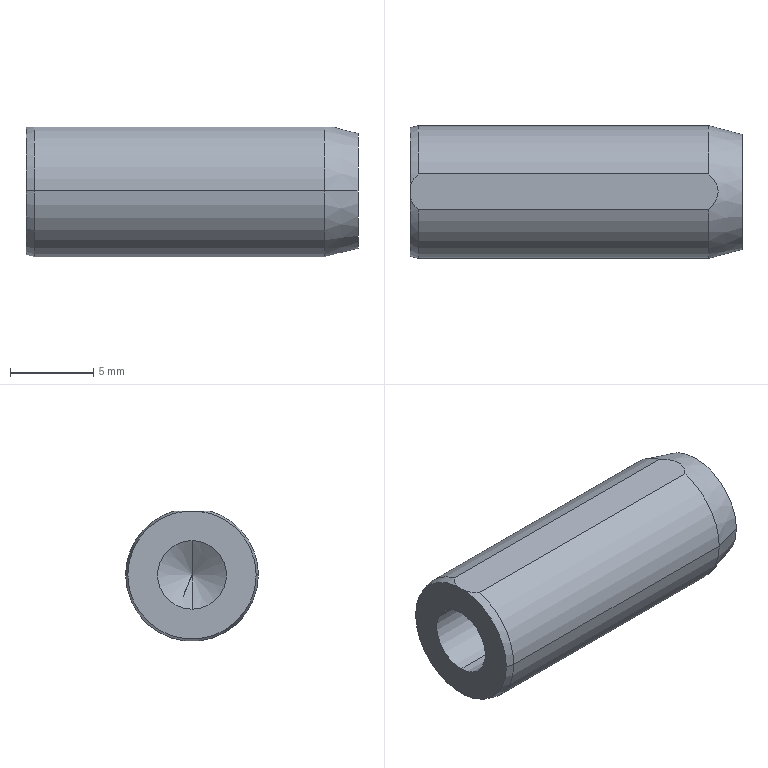Part | STEP file | MSTMS8-20-Part-1 | 1 solid | 15 faces | box 20 x 8 x 7.85 mm | volume 874.766 mm3 | cone 7 | cylinder 5 | plane 3 | commonest cylinder face diameters 8 x3 4.134 x2
STEP:
#1=CARTESIAN_POINT('',(0.,0.,0.));
#2=DIRECTION('',(0.,0.,1.));
#3=DIRECTION('',(1.,0.,0.));
#4=AXIS2_PLACEMENT_3D('',#1,#2,#3);
#5=CARTESIAN_POINT('',(-26.,-265.,-87.933));
#6=VERTEX_POINT('',#5);
#7=CARTESIAN_POINT('',(-34.,-265.,-87.933));
#8=VERTEX_POINT('',#7);
#9=CARTESIAN_POINT('',(-34.,-265.,-87.933));
#10=DIRECTION('',(-1.,0.,0.));
#11=VECTOR('',#10,1.);
#12=LINE('',#9,#11);
#13=CARTESIAN_POINT('',(-34.,-265.,-90.));
#14=DIRECTION('',(-1.,0.,0.));
#15=DIRECTION('',(0.,0.,1.));
#16=AXIS2_PLACEMENT_3D('',#13,#14,#15);
#17=CYLINDRICAL_SURFACE('',#16,2.067);
#18=CARTESIAN_POINT('',(6.283,0.));
#19=DIRECTION('',(0.,1.));
#20=VECTOR('',#19,1.);
#21=LINE('',#18,#20);
#22=(GEOMETRIC_REPRESENTATION_CONTEXT(2)PARAMETRIC_REPRESENTATION_CONTEXT()REPRESENTATION_CONTEXT('',''));
#23=DEFINITIONAL_REPRESENTATION('',(#21),#22);
#24=PCURVE('',#17,#23);
#25=CARTESIAN_POINT('',(-34.,-265.,-90.));
#26=DIRECTION('',(-1.,0.,0.));
#27=DIRECTION('',(0.,0.,1.));
#28=AXIS2_PLACEMENT_3D('',#25,#26,#27);
#29=CYLINDRICAL_SURFACE('',#28,2.067);
#30=CARTESIAN_POINT('',(0.,0.));
#31=DIRECTION('',(0.,1.));
#32=VECTOR('',#31,1.);
#33=LINE('',#30,#32);
#34=(GEOMETRIC_REPRESENTATION_CONTEXT(2)PARAMETRIC_REPRESENTATION_CONTEXT()REPRESENTATION_CONTEXT('',''));
#35=DEFINITIONAL_REPRESENTATION('',(#33),#34);
#36=PCURVE('',#29,#35);
#37=SURFACE_CURVE('',#12,(#24,#36),.PCURVE_S1.);
#38=EDGE_CURVE('',#6,#8,#37,.T.);
#39=ORIENTED_EDGE('',*,*,#38,.T.);
#40=CARTESIAN_POINT('',(-34.,-265.,-92.067));
#41=VERTEX_POINT('',#40);
#42=CARTESIAN_POINT('',(-34.,-265.,-90.));
#43=DIRECTION('',(-1.,0.,0.));
#44=DIRECTION('',(0.,0.,1.));
#45=AXIS2_PLACEMENT_3D('',#42,#43,#44);
#46=CIRCLE('',#45,2.067);
#47=CARTESIAN_POINT('',(0.,0.));
#48=DIRECTION('',(1.,0.));
#49=VECTOR('',#48,1.);
#50=LINE('',#47,#49);
#51=(GEOMETRIC_REPRESENTATION_CONTEXT(2)PARAMETRIC_REPRESENTATION_CONTEXT()REPRESENTATION_CONTEXT('',''));
#52=DEFINITIONAL_REPRESENTATION('',(#50),#51);
#53=PCURVE('',#17,#52);
#54=CARTESIAN_POINT('',(-34.,-265.,-90.));
#55=DIRECTION('',(-1.,0.,0.));
#56=DIRECTION('',(0.,-1.,0.));
#57=AXIS2_PLACEMENT_3D('',#54,#55,#56);
#58=PLANE('',#57);
#59=CARTESIAN_POINT('',(0.,0.));
#60=DIRECTION('',(0.,1.));
#61=AXIS2_PLACEMENT_2D('',#59,#60);
#62=CIRCLE('',#61,2.067);
#63=(GEOMETRIC_REPRESENTATION_CONTEXT(2)PARAMETRIC_REPRESENTATION_CONTEXT()REPRESENTATION_CONTEXT('',''));
#64=DEFINITIONAL_REPRESENTATION('',(#62),#63);
#65=PCURVE('',#58,#64);
#66=SURFACE_CURVE('',#46,(#53,#65),.PCURVE_S1.);
#67=EDGE_CURVE('',#41,#8,#66,.T.);
#68=ORIENTED_EDGE('',*,*,#67,.F.);
#69=CARTESIAN_POINT('',(-26.,-265.,-92.067));
#70=VERTEX_POINT('',#69);
#71=CARTESIAN_POINT('',(-34.,-265.,-92.067));
#72=DIRECTION('',(-1.,0.,0.));
#73=VECTOR('',#72,1.);
#74=LINE('',#71,#73);
#75=CARTESIAN_POINT('',(3.142,0.));
#76=DIRECTION('',(0.,1.));
#77=VECTOR('',#76,1.);
#78=LINE('',#75,#77);
#79=(GEOMETRIC_REPRESENTATION_CONTEXT(2)PARAMETRIC_REPRESENTATION_CONTEXT()REPRESENTATION_CONTEXT('',''));
#80=DEFINITIONAL_REPRESENTATION('',(#78),#79);
#81=PCURVE('',#17,#80);
#82=CARTESIAN_POINT('',(3.142,0.));
#83=DIRECTION('',(0.,1.));
#84=VECTOR('',#83,1.);
#85=LINE('',#82,#84);
#86=(GEOMETRIC_REPRESENTATION_CONTEXT(2)PARAMETRIC_REPRESENTATION_CONTEXT()REPRESENTATION_CONTEXT('',''));
#87=DEFINITIONAL_REPRESENTATION('',(#85),#86);
#88=PCURVE('',#29,#87);
#89=SURFACE_CURVE('',#74,(#81,#88),.PCURVE_S1.);
#90=EDGE_CURVE('',#70,#41,#89,.T.);
#91=ORIENTED_EDGE('',*,*,#90,.F.);
#92=CARTESIAN_POINT('',(-26.,-265.,-90.));
#93=DIRECTION('',(-1.,0.,0.));
#94=DIRECTION('',(0.,0.,1.));
#95=AXIS2_PLACEMENT_3D('',#92,#93,#94);
#96=CIRCLE('',#95,2.067);
#97=CARTESIAN_POINT('',(0.,-8.));
#98=DIRECTION('',(1.,0.));
#99=VECTOR('',#98,1.);
#100=LINE('',#97,#99);
#101=(GEOMETRIC_REPRESENTATION_CONTEXT(2)PARAMETRIC_REPRESENTATION_CONTEXT()REPRESENTATION_CONTEXT('',''));
#102=DEFINITIONAL_REPRESENTATION('',(#100),#101);
#103=PCURVE('',#17,#102);
#104=CARTESIAN_POINT('',(-26.,-265.,-90.));
#105=DIRECTION('',(-1.,0.,0.));
#106=DIRECTION('',(0.,0.,1.));
#107=AXIS2_PLACEMENT_3D('',#104,#105,#106);
#108=CONICAL_SURFACE('',#107,2.067,1.03);
#109=CARTESIAN_POINT('',(0.,0.));
#110=DIRECTION('',(1.,0.));
#111=VECTOR('',#110,1.);
#112=LINE('',#109,#111);
#113=(GEOMETRIC_REPRESENTATION_CONTEXT(2)PARAMETRIC_REPRESENTATION_CONTEXT()REPRESENTATION_CONTEXT('',''));
#114=DEFINITIONAL_REPRESENTATION('',(#112),#113);
#115=PCURVE('',#108,#114);
#116=SURFACE_CURVE('',#96,(#103,#115),.PCURVE_S1.);
#117=EDGE_CURVE('',#70,#6,#116,.T.);
#118=ORIENTED_EDGE('',*,*,#117,.T.);
#119=EDGE_LOOP('',(#39,#68,#91,#118));
#120=FACE_BOUND('',#119,.F.);
#121=ADVANCED_FACE('',(#120),#17,.F.);
#122=ORIENTED_EDGE('',*,*,#117,.F.);
#123=CARTESIAN_POINT('',(-24.758,-265.,-90.));
#124=VERTEX_POINT('',#123);
#125=CARTESIAN_POINT('',(-26.,-265.,-92.067));
#126=DIRECTION('',(-0.515,0.,-0.8572));
#127=VECTOR('',#126,1.);
#128=LINE('',#125,#127);
#129=CARTESIAN_POINT('',(3.142,0.));
#130=DIRECTION('',(0.,1.));
#131=VECTOR('',#130,1.);
#132=LINE('',#129,#131);
#133=(GEOMETRIC_REPRESENTATION_CONTEXT(2)PARAMETRIC_REPRESENTATION_CONTEXT()REPRESENTATION_CONTEXT('',''));
#134=DEFINITIONAL_REPRESENTATION('',(#132),#133);
#135=PCURVE('',#108,#134);
#136=CARTESIAN_POINT('',(-26.,-265.,-90.));
#137=DIRECTION('',(-1.,0.,0.));
#138=DIRECTION('',(0.,0.,1.));
#139=AXIS2_PLACEMENT_3D('',#136,#137,#138);
#140=CONICAL_SURFACE('',#139,2.067,1.03);
#141=CARTESIAN_POINT('',(3.142,0.));
#142=DIRECTION('',(0.,1.));
#143=VECTOR('',#142,1.);
#144=LINE('',#141,#143);
#145=(GEOMETRIC_REPRESENTATION_CONTEXT(2)PARAMETRIC_REPRESENTATION_CONTEXT()REPRESENTATION_CONTEXT('',''));
#146=DEFINITIONAL_REPRESENTATION('',(#144),#145);
#147=PCURVE('',#140,#146);
#148=SURFACE_CURVE('',#128,(#135,#147),.PCURVE_S1.);
#149=EDGE_CURVE('',#124,#70,#148,.T.);
#150=ORIENTED_EDGE('',*,*,#149,.F.);
#151=CARTESIAN_POINT('',(-26.,-265.,-87.933));
#152=DIRECTION('',(-0.515,0.,0.8572));
#153=VECTOR('',#152,1.);
#154=LINE('',#151,#153);
#155=CARTESIAN_POINT('',(6.283,0.));
#156=DIRECTION('',(0.,1.));
#157=VECTOR('',#156,1.);
#158=LINE('',#155,#157);
#159=(GEOMETRIC_REPRESENTATION_CONTEXT(2)PARAMETRIC_REPRESENTATION_CONTEXT()REPRESENTATION_CONTEXT('',''));
#160=DEFINITIONAL_REPRESENTATION('',(#158),#159);
#161=PCURVE('',#108,#160);
#162=CARTESIAN_POINT('',(0.,0.));
#163=DIRECTION('',(0.,1.));
#164=VECTOR('',#163,1.);
#165=LINE('',#162,#164);
#166=(GEOMETRIC_REPRESENTATION_CONTEXT(2)PARAMETRIC_REPRESENTATION_CONTEXT()REPRESENTATION_CONTEXT('',''));
#167=DEFINITIONAL_REPRESENTATION('',(#165),#166);
#168=PCURVE('',#140,#167);
#169=SURFACE_CURVE('',#154,(#161,#168),.PCURVE_S1.);
#170=EDGE_CURVE('',#124,#6,#169,.T.);
#171=ORIENTED_EDGE('',*,*,#170,.T.);
#172=EDGE_LOOP('',(#122,#150,#171));
#173=FACE_BOUND('',#172,.F.);
#174=ADVANCED_FACE('',(#173),#108,.F.);
#175=CARTESIAN_POINT('',(-14.,-261.536,-90.));
#176=VERTEX_POINT('',#175);
#177=CARTESIAN_POINT('',(-14.,-268.464,-90.));
#178=VERTEX_POINT('',#177);
#179=CARTESIAN_POINT('',(-14.,-265.,-90.));
#180=DIRECTION('',(1.,0.,0.));
#181=DIRECTION('',(0.,1.,0.));
#182=AXIS2_PLACEMENT_3D('',#179,#180,#181);
#183=CIRCLE('',#182,3.464);
#184=CARTESIAN_POINT('',(-14.,-265.,-90.));
#185=DIRECTION('',(-1.,0.,0.));
#186=DIRECTION('',(0.,-1.,0.));
#187=AXIS2_PLACEMENT_3D('',#184,#185,#186);
#188=CONICAL_SURFACE('',#187,3.464,0.2618);
#189=CARTESIAN_POINT('',(3.142,0.));
#190=DIRECTION('',(-1.,0.));
#191=VECTOR('',#190,1.);
#192=LINE('',#189,#191);
#193=(GEOMETRIC_REPRESENTATION_CONTEXT(2)PARAMETRIC_REPRESENTATION_CONTEXT()REPRESENTATION_CONTEXT('',''));
#194=DEFINITIONAL_REPRESENTATION('',(#192),#193);
#195=PCURVE('',#188,#194);
#196=CARTESIAN_POINT('',(-14.,-265.,-90.));
#197=DIRECTION('',(1.,0.,0.));
#198=DIRECTION('',(0.,1.,0.));
#199=AXIS2_PLACEMENT_3D('',#196,#197,#198);
#200=PLANE('',#199);
#201=CARTESIAN_POINT('',(0.,0.));
#202=DIRECTION('',(1.,0.));
#203=AXIS2_PLACEMENT_2D('',#201,#202);
#204=CIRCLE('',#203,3.464);
#205=(GEOMETRIC_REPRESENTATION_CONTEXT(2)PARAMETRIC_REPRESENTATION_CONTEXT()REPRESENTATION_CONTEXT('',''));
#206=DEFINITIONAL_REPRESENTATION('',(#204),#205);
#207=PCURVE('',#200,#206);
#208=SURFACE_CURVE('',#183,(#195,#207),.PCURVE_S1.);
#209=EDGE_CURVE('',#176,#178,#208,.T.);
#210=ORIENTED_EDGE('',*,*,#209,.F.);
#211=CARTESIAN_POINT('',(-16.,-261.,-90.));
#212=VERTEX_POINT('',#211);
#213=CARTESIAN_POINT('',(-14.,-261.536,-90.));
#214=DIRECTION('',(-0.9659,0.2588,0.));
#215=VECTOR('',#214,1.);
#216=LINE('',#213,#215);
#217=CARTESIAN_POINT('',(3.142,0.));
#218=DIRECTION('',(0.,1.));
#219=VECTOR('',#218,1.);
#220=LINE('',#217,#219);
#221=(GEOMETRIC_REPRESENTATION_CONTEXT(2)PARAMETRIC_REPRESENTATION_CONTEXT()REPRESENTATION_CONTEXT('',''));
#222=DEFINITIONAL_REPRESENTATION('',(#220),#221);
#223=PCURVE('',#188,#222);
#224=CARTESIAN_POINT('',(-14.,-265.,-90.));
#225=DIRECTION('',(-1.,0.,0.));
#226=DIRECTION('',(0.,-1.,0.));
#227=AXIS2_PLACEMENT_3D('',#224,#225,#226);
#228=CONICAL_SURFACE('',#227,3.464,0.2618);
#229=CARTESIAN_POINT('',(3.142,0.));
#230=DIRECTION('',(0.,1.));
#231=VECTOR('',#230,1.);
#232=LINE('',#229,#231);
#233=(GEOMETRIC_REPRESENTATION_CONTEXT(2)PARAMETRIC_REPRESENTATION_CONTEXT()REPRESENTATION_CONTEXT('',''));
#234=DEFINITIONAL_REPRESENTATION('',(#232),#233);
#235=PCURVE('',#228,#234);
#236=SURFACE_CURVE('',#216,(#223,#235),.PCURVE_S1.);
#237=EDGE_CURVE('',#176,#212,#236,.T.);
#238=ORIENTED_EDGE('',*,*,#237,.T.);
#239=CARTESIAN_POINT('',(-16.,-263.915,-86.15));
#240=VERTEX_POINT('',#239);
#241=CARTESIAN_POINT('',(-16.,-265.,-90.));
#242=DIRECTION('',(1.,0.,0.));
#243=DIRECTION('',(0.,1.,0.));
#244=AXIS2_PLACEMENT_3D('',#241,#242,#243);
#245=CIRCLE('',#244,4.);
#246=CARTESIAN_POINT('',(3.142,2.));
#247=DIRECTION('',(-1.,0.));
#248=VECTOR('',#247,1.);
#249=LINE('',#246,#248);
#250=(GEOMETRIC_REPRESENTATION_CONTEXT(2)PARAMETRIC_REPRESENTATION_CONTEXT()REPRESENTATION_CONTEXT('',''));
#251=DEFINITIONAL_REPRESENTATION('',(#249),#250);
#252=PCURVE('',#188,#251);
#253=CARTESIAN_POINT('',(-14.,-265.,-90.));
#254=DIRECTION('',(1.,0.,0.));
#255=DIRECTION('',(0.,1.,0.));
#256=AXIS2_PLACEMENT_3D('',#253,#254,#255);
#257=CYLINDRICAL_SURFACE('',#256,4.);
#258=CARTESIAN_POINT('',(0.,-2.));
#259=DIRECTION('',(1.,0.));
#260=VECTOR('',#259,1.);
#261=LINE('',#258,#260);
#262=(GEOMETRIC_REPRESENTATION_CONTEXT(2)PARAMETRIC_REPRESENTATION_CONTEXT()REPRESENTATION_CONTEXT('',''));
#263=DEFINITIONAL_REPRESENTATION('',(#261),#262);
#264=PCURVE('',#257,#263);
#265=SURFACE_CURVE('',#245,(#252,#264),.PCURVE_S1.);
#266=EDGE_CURVE('',#212,#240,#265,.T.);
#267=ORIENTED_EDGE('',*,*,#266,.T.);
#268=CARTESIAN_POINT('',(-16.,-266.085,-86.15));
#269=VERTEX_POINT('',#268);
#270=CARTESIAN_POINT('',(-16.,-266.085,-86.15));
#271=CARTESIAN_POINT('',(-15.853,-265.94,-86.15));
#272=CARTESIAN_POINT('',(-15.716,-265.778,-86.15));
#273=CARTESIAN_POINT('',(-15.508,-265.416,-86.15));
#274=CARTESIAN_POINT('',(-15.44,-265.21,-86.15));
#275=CARTESIAN_POINT('',(-15.44,-264.789,-86.15));
#276=CARTESIAN_POINT('',(-15.508,-264.584,-86.15));
#277=CARTESIAN_POINT('',(-15.663,-264.313,-86.15));
#278=CARTESIAN_POINT('',(-15.724,-264.227,-86.15));
#279=CARTESIAN_POINT('',(-15.856,-264.064,-86.15));
#280=CARTESIAN_POINT('',(-15.926,-263.988,-86.15));
#281=CARTESIAN_POINT('',(-16.,-263.915,-86.15));
#282=B_SPLINE_CURVE_WITH_KNOTS('',3,(#270,#271,#272,#273,#274,#275,#276,#277,#278,#279,#280,#281),.UNSPECIFIED.,.F.,.F.,(4,2,2,2,2,4),(0.001238,0.001854,0.00247,0.003086,0.003394,0.003702),.UNSPECIFIED.);
#283=CARTESIAN_POINT('',(1.296,2.));
#284=CARTESIAN_POINT('',(1.302,1.973));
#285=CARTESIAN_POINT('',(1.315,1.921));
#286=CARTESIAN_POINT('',(1.336,1.844));
#287=CARTESIAN_POINT('',(1.358,1.771));
#288=CARTESIAN_POINT('',(1.38,1.703));
#289=CARTESIAN_POINT('',(1.404,1.64));
#290=CARTESIAN_POINT('',(1.429,1.583));
#291=CARTESIAN_POINT('',(1.456,1.534));
#292=CARTESIAN_POINT('',(1.483,1.494));
#293=CARTESIAN_POINT('',(1.512,1.464));
#294=CARTESIAN_POINT('',(1.541,1.445));
#295=CARTESIAN_POINT('',(1.571,1.438));
#296=CARTESIAN_POINT('',(1.601,1.445));
#297=CARTESIAN_POINT('',(1.63,1.464));
#298=CARTESIAN_POINT('',(1.658,1.494));
#299=CARTESIAN_POINT('',(1.686,1.534));
#300=CARTESIAN_POINT('',(1.712,1.583));
#301=CARTESIAN_POINT('',(1.737,1.64));
#302=CARTESIAN_POINT('',(1.761,1.703));
#303=CARTESIAN_POINT('',(1.784,1.772));
#304=CARTESIAN_POINT('',(1.806,1.844));
#305=CARTESIAN_POINT('',(1.826,1.92));
#306=CARTESIAN_POINT('',(1.839,1.973));
#307=CARTESIAN_POINT('',(1.846,2.));
#308=B_SPLINE_CURVE_WITH_KNOTS('',3,(#283,#284,#285,#286,#287,#288,#289,#290,#291,#292,#293,#294,#295,#296,#297,#298,#299,#300,#301,#302,#303,#304,#305,#306,#307),.UNSPECIFIED.,.F.,.F.,(4,1,1,1,1,1,1,1,1,1,1,1,1,1,1,1,1,1,1,1,1,1,4),(0.001238,0.00135,0.001462,0.001574,0.001686,0.001798,0.00191,0.002022,0.002134,0.002246,0.002358,0.00247,0.002582,0.002694,0.002806,0.002918,0.00303,0.003142,0.003254,0.003366,0.003478,0.00359,0.003702),.QUASI_UNIFORM_KNOTS.);
#309=(GEOMETRIC_REPRESENTATION_CONTEXT(2)PARAMETRIC_REPRESENTATION_CONTEXT()REPRESENTATION_CONTEXT('',''));
#310=DEFINITIONAL_REPRESENTATION('',(#308),#309);
#311=PCURVE('',#188,#310);
#312=CARTESIAN_POINT('',(-34.,-263.915,-86.15));
#313=DIRECTION('',(0.,0.,-1.));
#314=DIRECTION('',(-1.,0.,0.));
#315=AXIS2_PLACEMENT_3D('',#312,#313,#314);
#316=PLANE('',#315);
#317=CARTESIAN_POINT('',(-18.,-2.17));
#318=CARTESIAN_POINT('',(-18.147,-2.025));
#319=CARTESIAN_POINT('',(-18.284,-1.864));
#320=CARTESIAN_POINT('',(-18.492,-1.501));
#321=CARTESIAN_POINT('',(-18.56,-1.295));
#322=CARTESIAN_POINT('',(-18.56,-0.8744));
#323=CARTESIAN_POINT('',(-18.492,-0.6696));
#324=CARTESIAN_POINT('',(-18.337,-0.3981));
#325=CARTESIAN_POINT('',(-18.276,-0.3116));
#326=CARTESIAN_POINT('',(-18.144,-0.1493));
#327=CARTESIAN_POINT('',(-18.074,-0.07297));
#328=CARTESIAN_POINT('',(-18.,0.));
#329=B_SPLINE_CURVE_WITH_KNOTS('',3,(#317,#318,#319,#320,#321,#322,#323,#324,#325,#326,#327,#328),.UNSPECIFIED.,.F.,.F.,(4,2,2,2,2,4),(0.001238,0.001854,0.00247,0.003086,0.003394,0.003702),.UNSPECIFIED.);
#330=(GEOMETRIC_REPRESENTATION_CONTEXT(2)PARAMETRIC_REPRESENTATION_CONTEXT()REPRESENTATION_CONTEXT('',''));
#331=DEFINITIONAL_REPRESENTATION('',(#329),#330);
#332=PCURVE('',#316,#331);
#333=SURFACE_CURVE('',#282,(#311,#332),.PCURVE_S1.);
#334=EDGE_CURVE('',#269,#240,#333,.T.);
#335=ORIENTED_EDGE('',*,*,#334,.F.);
#336=CARTESIAN_POINT('',(-16.,-269.,-90.));
#337=VERTEX_POINT('',#336);
#338=CARTESIAN_POINT('',(-16.,-265.,-90.));
#339=DIRECTION('',(1.,0.,0.));
#340=DIRECTION('',(0.,1.,0.));
#341=AXIS2_PLACEMENT_3D('',#338,#339,#340);
#342=CIRCLE('',#341,4.);
#343=CARTESIAN_POINT('',(3.142,2.));
#344=DIRECTION('',(-1.,0.));
#345=VECTOR('',#344,1.);
#346=LINE('',#343,#345);
#347=(GEOMETRIC_REPRESENTATION_CONTEXT(2)PARAMETRIC_REPRESENTATION_CONTEXT()REPRESENTATION_CONTEXT('',''));
#348=DEFINITIONAL_REPRESENTATION('',(#346),#347);
#349=PCURVE('',#188,#348);
#350=CARTESIAN_POINT('',(-14.,-265.,-90.));
#351=DIRECTION('',(1.,0.,0.));
#352=DIRECTION('',(0.,1.,0.));
#353=AXIS2_PLACEMENT_3D('',#350,#351,#352);
#354=CYLINDRICAL_SURFACE('',#353,4.);
#355=CARTESIAN_POINT('',(0.,-2.));
#356=DIRECTION('',(1.,0.));
#357=VECTOR('',#356,1.);
#358=LINE('',#355,#357);
#359=(GEOMETRIC_REPRESENTATION_CONTEXT(2)PARAMETRIC_REPRESENTATION_CONTEXT()REPRESENTATION_CONTEXT('',''));
#360=DEFINITIONAL_REPRESENTATION('',(#358),#359);
#361=PCURVE('',#354,#360);
#362=SURFACE_CURVE('',#342,(#349,#361),.PCURVE_S1.);
#363=EDGE_CURVE('',#269,#337,#362,.T.);
#364=ORIENTED_EDGE('',*,*,#363,.T.);
#365=CARTESIAN_POINT('',(-14.,-268.464,-90.));
#366=DIRECTION('',(-0.9659,-0.2588,0.));
#367=VECTOR('',#366,1.);
#368=LINE('',#365,#367);
#369=CARTESIAN_POINT('',(0.,0.));
#370=DIRECTION('',(0.,1.));
#371=VECTOR('',#370,1.);
#372=LINE('',#369,#371);
#373=(GEOMETRIC_REPRESENTATION_CONTEXT(2)PARAMETRIC_REPRESENTATION_CONTEXT()REPRESENTATION_CONTEXT('',''));
#374=DEFINITIONAL_REPRESENTATION('',(#372),#373);
#375=PCURVE('',#188,#374);
#376=CARTESIAN_POINT('',(6.283,0.));
#377=DIRECTION('',(0.,1.));
#378=VECTOR('',#377,1.);
#379=LINE('',#376,#378);
#380=(GEOMETRIC_REPRESENTATION_CONTEXT(2)PARAMETRIC_REPRESENTATION_CONTEXT()REPRESENTATION_CONTEXT('',''));
#381=DEFINITIONAL_REPRESENTATION('',(#379),#380);
#382=PCURVE('',#228,#381);
#383=SURFACE_CURVE('',#368,(#375,#382),.PCURVE_S1.);
#384=EDGE_CURVE('',#178,#337,#383,.T.);
#385=ORIENTED_EDGE('',*,*,#384,.F.);
#386=EDGE_LOOP('',(#210,#238,#267,#335,#364,#385));
#387=FACE_BOUND('',#386,.T.);
#388=ADVANCED_FACE('',(#387),#188,.T.);
#389=CARTESIAN_POINT('',(-33.5,-266.085,-86.15));
#390=VERTEX_POINT('',#389);
#391=CARTESIAN_POINT('',(-33.5,-269.,-90.));
#392=VERTEX_POINT('',#391);
#393=CARTESIAN_POINT('',(-33.5,-265.,-90.));
#394=DIRECTION('',(1.,0.,0.));
#395=DIRECTION('',(0.,1.,0.));
#396=AXIS2_PLACEMENT_3D('',#393,#394,#395);
#397=CIRCLE('',#396,4.);
#398=CARTESIAN_POINT('',(0.,-19.5));
#399=DIRECTION('',(1.,0.));
#400=VECTOR('',#399,1.);
#401=LINE('',#398,#400);
#402=(GEOMETRIC_REPRESENTATION_CONTEXT(2)PARAMETRIC_REPRESENTATION_CONTEXT()REPRESENTATION_CONTEXT('',''));
#403=DEFINITIONAL_REPRESENTATION('',(#401),#402);
#404=PCURVE('',#354,#403);
#405=CARTESIAN_POINT('',(-33.5,-265.,-90.));
#406=DIRECTION('',(1.,0.,0.));
#407=DIRECTION('',(0.,1.,0.));
#408=AXIS2_PLACEMENT_3D('',#405,#406,#407);
#409=CONICAL_SURFACE('',#408,4.,0.2618);
#410=CARTESIAN_POINT('',(0.,0.));
#411=DIRECTION('',(1.,0.));
#412=VECTOR('',#411,1.);
#413=LINE('',#410,#412);
#414=(GEOMETRIC_REPRESENTATION_CONTEXT(2)PARAMETRIC_REPRESENTATION_CONTEXT()REPRESENTATION_CONTEXT('',''));
#415=DEFINITIONAL_REPRESENTATION('',(#413),#414);
#416=PCURVE('',#409,#415);
#417=SURFACE_CURVE('',#397,(#404,#416),.PCURVE_S1.);
#418=EDGE_CURVE('',#390,#392,#417,.T.);
#419=ORIENTED_EDGE('',*,*,#418,.T.);
#420=CARTESIAN_POINT('',(-14.,-269.,-90.));
#421=DIRECTION('',(1.,0.,0.));
#422=VECTOR('',#421,1.);
#423=LINE('',#420,#422);
#424=CARTESIAN_POINT('',(3.142,0.));
#425=DIRECTION('',(0.,1.));
#426=VECTOR('',#425,1.);
#427=LINE('',#424,#426);
#428=(GEOMETRIC_REPRESENTATION_CONTEXT(2)PARAMETRIC_REPRESENTATION_CONTEXT()REPRESENTATION_CONTEXT('',''));
#429=DEFINITIONAL_REPRESENTATION('',(#427),#428);
#430=PCURVE('',#354,#429);
#431=CARTESIAN_POINT('',(-14.,-265.,-90.));
#432=DIRECTION('',(1.,0.,0.));
#433=DIRECTION('',(0.,1.,0.));
#434=AXIS2_PLACEMENT_3D('',#431,#432,#433);
#435=CYLINDRICAL_SURFACE('',#434,4.);
#436=CARTESIAN_POINT('',(3.142,0.));
#437=DIRECTION('',(0.,1.));
#438=VECTOR('',#437,1.);
#439=LINE('',#436,#438);
#440=(GEOMETRIC_REPRESENTATION_CONTEXT(2)PARAMETRIC_REPRESENTATION_CONTEXT()REPRESENTATION_CONTEXT('',''));
#441=DEFINITIONAL_REPRESENTATION('',(#439),#440);
#442=PCURVE('',#435,#441);
#443=SURFACE_CURVE('',#423,(#430,#442),.PCURVE_S1.);
#444=EDGE_CURVE('',#392,#337,#443,.T.);
#445=ORIENTED_EDGE('',*,*,#444,.T.);
#446=ORIENTED_EDGE('',*,*,#363,.F.);
#447=CARTESIAN_POINT('',(-34.,-266.085,-86.15));
#448=DIRECTION('',(1.,0.,0.));
#449=VECTOR('',#448,1.);
#450=LINE('',#447,#449);
#451=CARTESIAN_POINT('',(1.846,-20.));
#452=DIRECTION('',(0.,1.));
#453=VECTOR('',#452,1.);
#454=LINE('',#451,#453);
#455=(GEOMETRIC_REPRESENTATION_CONTEXT(2)PARAMETRIC_REPRESENTATION_CONTEXT()REPRESENTATION_CONTEXT('',''));
#456=DEFINITIONAL_REPRESENTATION('',(#454),#455);
#457=PCURVE('',#354,#456);
#458=CARTESIAN_POINT('',(0.,-2.17));
#459=DIRECTION('',(-1.,0.));
#460=VECTOR('',#459,1.);
#461=LINE('',#458,#460);
#462=(GEOMETRIC_REPRESENTATION_CONTEXT(2)PARAMETRIC_REPRESENTATION_CONTEXT()REPRESENTATION_CONTEXT('',''));
#463=DEFINITIONAL_REPRESENTATION('',(#461),#462);
#464=PCURVE('',#316,#463);
#465=SURFACE_CURVE('',#450,(#457,#464),.PCURVE_S1.);
#466=EDGE_CURVE('',#390,#269,#465,.T.);
#467=ORIENTED_EDGE('',*,*,#466,.F.);
#468=EDGE_LOOP('',(#419,#445,#446,#467));
#469=FACE_BOUND('',#468,.T.);
#470=ADVANCED_FACE('',(#469),#354,.T.);
#471=ORIENTED_EDGE('',*,*,#444,.F.);
#472=CARTESIAN_POINT('',(-33.5,-261.,-90.));
#473=VERTEX_POINT('',#472);
#474=CARTESIAN_POINT('',(-33.5,-265.,-90.));
#475=DIRECTION('',(1.,0.,0.));
#476=DIRECTION('',(0.,1.,0.));
#477=AXIS2_PLACEMENT_3D('',#474,#475,#476);
#478=CIRCLE('',#477,4.);
#479=CARTESIAN_POINT('',(0.,-19.5));
#480=DIRECTION('',(1.,0.));
#481=VECTOR('',#480,1.);
#482=LINE('',#479,#481);
#483=(GEOMETRIC_REPRESENTATION_CONTEXT(2)PARAMETRIC_REPRESENTATION_CONTEXT()REPRESENTATION_CONTEXT('',''));
#484=DEFINITIONAL_REPRESENTATION('',(#482),#483);
#485=PCURVE('',#435,#484);
#486=CARTESIAN_POINT('',(-33.5,-265.,-90.));
#487=DIRECTION('',(1.,0.,0.));
#488=DIRECTION('',(0.,1.,0.));
#489=AXIS2_PLACEMENT_3D('',#486,#487,#488);
#490=CONICAL_SURFACE('',#489,4.,0.2618);
#491=CARTESIAN_POINT('',(0.,0.));
#492=DIRECTION('',(1.,0.));
#493=VECTOR('',#492,1.);
#494=LINE('',#491,#493);
#495=(GEOMETRIC_REPRESENTATION_CONTEXT(2)PARAMETRIC_REPRESENTATION_CONTEXT()REPRESENTATION_CONTEXT('',''));
#496=DEFINITIONAL_REPRESENTATION('',(#494),#495);
#497=PCURVE('',#490,#496);
#498=SURFACE_CURVE('',#478,(#485,#497),.PCURVE_S1.);
#499=EDGE_CURVE('',#392,#473,#498,.T.);
#500=ORIENTED_EDGE('',*,*,#499,.T.);
#501=CARTESIAN_POINT('',(-14.,-261.,-90.));
#502=DIRECTION('',(1.,0.,0.));
#503=VECTOR('',#502,1.);
#504=LINE('',#501,#503);
#505=CARTESIAN_POINT('',(6.283,0.));
#506=DIRECTION('',(0.,1.));
#507=VECTOR('',#506,1.);
#508=LINE('',#505,#507);
#509=(GEOMETRIC_REPRESENTATION_CONTEXT(2)PARAMETRIC_REPRESENTATION_CONTEXT()REPRESENTATION_CONTEXT('',''));
#510=DEFINITIONAL_REPRESENTATION('',(#508),#509);
#511=PCURVE('',#435,#510);
#512=CARTESIAN_POINT('',(0.,0.));
#513=DIRECTION('',(0.,1.));
#514=VECTOR('',#513,1.);
#515=LINE('',#512,#514);
#516=(GEOMETRIC_REPRESENTATION_CONTEXT(2)PARAMETRIC_REPRESENTATION_CONTEXT()REPRESENTATION_CONTEXT('',''));
#517=DEFINITIONAL_REPRESENTATION('',(#515),#516);
#518=PCURVE('',#257,#517);
#519=SURFACE_CURVE('',#504,(#511,#518),.PCURVE_S1.);
#520=EDGE_CURVE('',#473,#212,#519,.T.);
#521=ORIENTED_EDGE('',*,*,#520,.T.);
#522=CARTESIAN_POINT('',(-16.,-265.,-90.));
#523=DIRECTION('',(1.,0.,0.));
#524=DIRECTION('',(0.,1.,0.));
#525=AXIS2_PLACEMENT_3D('',#522,#523,#524);
#526=CIRCLE('',#525,4.);
#527=CARTESIAN_POINT('',(0.,-2.));
#528=DIRECTION('',(1.,0.));
#529=VECTOR('',#528,1.);
#530=LINE('',#527,#529);
#531=(GEOMETRIC_REPRESENTATION_CONTEXT(2)PARAMETRIC_REPRESENTATION_CONTEXT()REPRESENTATION_CONTEXT('',''));
#532=DEFINITIONAL_REPRESENTATION('',(#530),#531);
#533=PCURVE('',#435,#532);
#534=CARTESIAN_POINT('',(9.425,2.));
#535=DIRECTION('',(-1.,0.));
#536=VECTOR('',#535,1.);
#537=LINE('',#534,#536);
#538=(GEOMETRIC_REPRESENTATION_CONTEXT(2)PARAMETRIC_REPRESENTATION_CONTEXT()REPRESENTATION_CONTEXT('',''));
#539=DEFINITIONAL_REPRESENTATION('',(#537),#538);
#540=PCURVE('',#228,#539);
#541=SURFACE_CURVE('',#526,(#533,#540),.PCURVE_S1.);
#542=EDGE_CURVE('',#337,#212,#541,.T.);
#543=ORIENTED_EDGE('',*,*,#542,.F.);
#544=EDGE_LOOP('',(#471,#500,#521,#543));
#545=FACE_BOUND('',#544,.T.);
#546=ADVANCED_FACE('',(#545),#435,.T.);
#547=CARTESIAN_POINT('',(-34.,-265.352,-86.15));
#548=VERTEX_POINT('',#547);
#549=CARTESIAN_POINT('',(-34.,-268.866,-90.));
#550=VERTEX_POINT('',#549);
#551=CARTESIAN_POINT('',(-34.,-265.,-90.));
#552=DIRECTION('',(1.,0.,0.));
#553=DIRECTION('',(0.,1.,0.));
#554=AXIS2_PLACEMENT_3D('',#551,#552,#553);
#555=CIRCLE('',#554,3.866);
#556=CARTESIAN_POINT('',(0.,-0.5));
#557=DIRECTION('',(1.,0.));
#558=VECTOR('',#557,1.);
#559=LINE('',#556,#558);
#560=(GEOMETRIC_REPRESENTATION_CONTEXT(2)PARAMETRIC_REPRESENTATION_CONTEXT()REPRESENTATION_CONTEXT('',''));
#561=DEFINITIONAL_REPRESENTATION('',(#559),#560);
#562=PCURVE('',#409,#561);
#563=CARTESIAN_POINT('',(-3.866,0.));
#564=CARTESIAN_POINT('',(-3.866,6.696));
#565=CARTESIAN_POINT('',(1.933,3.348));
#566=CARTESIAN_POINT('',(7.732,0.));
#567=CARTESIAN_POINT('',(1.933,-3.348));
#568=CARTESIAN_POINT('',(-3.866,-6.696));
#569=CARTESIAN_POINT('',(-3.866,0.));
#570=(BOUNDED_CURVE()B_SPLINE_CURVE(2,(#563,#564,#565,#566,#567,#568,#569),.UNSPECIFIED.,.T.,.F.)B_SPLINE_CURVE_WITH_KNOTS((1,2,2,2,2,1),(-2.094,0.,2.094,4.189,6.283,8.378),.UNSPECIFIED.)CURVE()GEOMETRIC_REPRESENTATION_ITEM()RATIONAL_B_SPLINE_CURVE((1.,0.5,1.,0.5,1.,0.5,1.))REPRESENTATION_ITEM(''));
#571=(GEOMETRIC_REPRESENTATION_CONTEXT(2)PARAMETRIC_REPRESENTATION_CONTEXT()REPRESENTATION_CONTEXT('',''));
#572=DEFINITIONAL_REPRESENTATION('',(#570),#571);
#573=PCURVE('',#58,#572);
#574=SURFACE_CURVE('',#555,(#562,#573),.PCURVE_S1.);
#575=EDGE_CURVE('',#548,#550,#574,.T.);
#576=ORIENTED_EDGE('',*,*,#575,.T.);
#577=CARTESIAN_POINT('',(-33.5,-269.,-90.));
#578=DIRECTION('',(0.9659,-0.2588,0.));
#579=VECTOR('',#578,1.);
#580=LINE('',#577,#579);
#581=CARTESIAN_POINT('',(3.142,0.));
#582=DIRECTION('',(0.,1.));
#583=VECTOR('',#582,1.);
#584=LINE('',#581,#583);
#585=(GEOMETRIC_REPRESENTATION_CONTEXT(2)PARAMETRIC_REPRESENTATION_CONTEXT()REPRESENTATION_CONTEXT('',''));
#586=DEFINITIONAL_REPRESENTATION('',(#584),#585);
#587=PCURVE('',#409,#586);
#588=CARTESIAN_POINT('',(3.142,0.));
#589=DIRECTION('',(0.,1.));
#590=VECTOR('',#589,1.);
#591=LINE('',#588,#590);
#592=(GEOMETRIC_REPRESENTATION_CONTEXT(2)PARAMETRIC_REPRESENTATION_CONTEXT()REPRESENTATION_CONTEXT('',''));
#593=DEFINITIONAL_REPRESENTATION('',(#591),#592);
#594=PCURVE('',#490,#593);
#595=SURFACE_CURVE('',#580,(#587,#594),.PCURVE_S1.);
#596=EDGE_CURVE('',#550,#392,#595,.T.);
#597=ORIENTED_EDGE('',*,*,#596,.T.);
#598=ORIENTED_EDGE('',*,*,#418,.F.);
#599=CARTESIAN_POINT('',(-34.,-265.352,-86.15));
#600=CARTESIAN_POINT('',(-33.952,-265.493,-86.15));
#601=CARTESIAN_POINT('',(-33.878,-265.626,-86.15));
#602=CARTESIAN_POINT('',(-33.706,-265.868,-86.15));
#603=CARTESIAN_POINT('',(-33.606,-265.98,-86.15));
#604=CARTESIAN_POINT('',(-33.5,-266.085,-86.15));
#605=B_SPLINE_CURVE_WITH_KNOTS('',3,(#599,#600,#601,#602,#603,#604),.UNSPECIFIED.,.F.,.F.,(4,2,4),(0.003237,0.003679,0.004122),.UNSPECIFIED.);
#606=CARTESIAN_POINT('',(1.662,-0.5));
#607=CARTESIAN_POINT('',(1.665,-0.4956));
#608=CARTESIAN_POINT('',(1.672,-0.4865));
#609=CARTESIAN_POINT('',(1.682,-0.4715));
#610=CARTESIAN_POINT('',(1.691,-0.4553));
#611=CARTESIAN_POINT('',(1.701,-0.4381));
#612=CARTESIAN_POINT('',(1.71,-0.4198));
#613=CARTESIAN_POINT('',(1.719,-0.4005));
#614=CARTESIAN_POINT('',(1.728,-0.3804));
#615=CARTESIAN_POINT('',(1.737,-0.3593));
#616=CARTESIAN_POINT('',(1.746,-0.3375));
#617=CARTESIAN_POINT('',(1.754,-0.315));
#618=CARTESIAN_POINT('',(1.763,-0.2918));
#619=CARTESIAN_POINT('',(1.771,-0.268));
#620=CARTESIAN_POINT('',(1.779,-0.2436));
#621=CARTESIAN_POINT('',(1.787,-0.2185));
#622=CARTESIAN_POINT('',(1.794,-0.1929));
#623=CARTESIAN_POINT('',(1.802,-0.1668));
#624=CARTESIAN_POINT('',(1.81,-0.1402));
#625=CARTESIAN_POINT('',(1.817,-0.113));
#626=CARTESIAN_POINT('',(1.824,-0.08541));
#627=CARTESIAN_POINT('',(1.832,-0.05736));
#628=CARTESIAN_POINT('',(1.839,-0.02891));
#629=CARTESIAN_POINT('',(1.843,-0.009676));
#630=CARTESIAN_POINT('',(1.846,0.));
#631=B_SPLINE_CURVE_WITH_KNOTS('',3,(#606,#607,#608,#609,#610,#611,#612,#613,#614,#615,#616,#617,#618,#619,#620,#621,#622,#623,#624,#625,#626,#627,#628,#629,#630),.UNSPECIFIED.,.F.,.F.,(4,1,1,1,1,1,1,1,1,1,1,1,1,1,1,1,1,1,1,1,1,1,4),(0.003237,0.003277,0.003317,0.003357,0.003398,0.003438,0.003478,0.003518,0.003559,0.003599,0.003639,0.003679,0.00372,0.00376,0.0038,0.00384,0.003881,0.003921,0.003961,0.004001,0.004042,0.004082,0.004122),.QUASI_UNIFORM_KNOTS.);
#632=(GEOMETRIC_REPRESENTATION_CONTEXT(2)PARAMETRIC_REPRESENTATION_CONTEXT()REPRESENTATION_CONTEXT('',''));
#633=DEFINITIONAL_REPRESENTATION('',(#631),#632);
#634=PCURVE('',#409,#633);
#635=CARTESIAN_POINT('',(0.,-1.437));
#636=CARTESIAN_POINT('',(-0.04803,-1.578));
#637=CARTESIAN_POINT('',(-0.1222,-1.711));
#638=CARTESIAN_POINT('',(-0.2944,-1.953));
#639=CARTESIAN_POINT('',(-0.3936,-2.065));
#640=CARTESIAN_POINT('',(-0.5,-2.17));
#641=B_SPLINE_CURVE_WITH_KNOTS('',3,(#635,#636,#637,#638,#639,#640),.UNSPECIFIED.,.F.,.F.,(4,2,4),(0.003237,0.003679,0.004122),.UNSPECIFIED.);
#642=(GEOMETRIC_REPRESENTATION_CONTEXT(2)PARAMETRIC_REPRESENTATION_CONTEXT()REPRESENTATION_CONTEXT('',''));
#643=DEFINITIONAL_REPRESENTATION('',(#641),#642);
#644=PCURVE('',#316,#643);
#645=SURFACE_CURVE('',#605,(#634,#644),.PCURVE_S1.);
#646=EDGE_CURVE('',#548,#390,#645,.T.);
#647=ORIENTED_EDGE('',*,*,#646,.F.);
#648=EDGE_LOOP('',(#576,#597,#598,#647));
#649=FACE_BOUND('',#648,.T.);
#650=ADVANCED_FACE('',(#649),#409,.T.);
#651=ORIENTED_EDGE('',*,*,#596,.F.);
#652=CARTESIAN_POINT('',(-34.,-261.134,-90.));
#653=VERTEX_POINT('',#652);
#654=CARTESIAN_POINT('',(-34.,-265.,-90.));
#655=DIRECTION('',(1.,0.,0.));
#656=DIRECTION('',(0.,1.,0.));
#657=AXIS2_PLACEMENT_3D('',#654,#655,#656);
#658=CIRCLE('',#657,3.866);
#659=CARTESIAN_POINT('',(0.,-0.5));
#660=DIRECTION('',(1.,0.));
#661=VECTOR('',#660,1.);
#662=LINE('',#659,#661);
#663=(GEOMETRIC_REPRESENTATION_CONTEXT(2)PARAMETRIC_REPRESENTATION_CONTEXT()REPRESENTATION_CONTEXT('',''));
#664=DEFINITIONAL_REPRESENTATION('',(#662),#663);
#665=PCURVE('',#490,#664);
#666=CARTESIAN_POINT('',(-3.866,0.));
#667=CARTESIAN_POINT('',(-3.866,6.696));
#668=CARTESIAN_POINT('',(1.933,3.348));
#669=CARTESIAN_POINT('',(7.732,0.));
#670=CARTESIAN_POINT('',(1.933,-3.348));
#671=CARTESIAN_POINT('',(-3.866,-6.696));
#672=CARTESIAN_POINT('',(-3.866,0.));
#673=(BOUNDED_CURVE()B_SPLINE_CURVE(2,(#666,#667,#668,#669,#670,#671,#672),.UNSPECIFIED.,.T.,.F.)B_SPLINE_CURVE_WITH_KNOTS((1,2,2,2,2,1),(-2.094,0.,2.094,4.189,6.283,8.378),.UNSPECIFIED.)CURVE()GEOMETRIC_REPRESENTATION_ITEM()RATIONAL_B_SPLINE_CURVE((1.,0.5,1.,0.5,1.,0.5,1.))REPRESENTATION_ITEM(''));
#674=(GEOMETRIC_REPRESENTATION_CONTEXT(2)PARAMETRIC_REPRESENTATION_CONTEXT()REPRESENTATION_CONTEXT('',''));
#675=DEFINITIONAL_REPRESENTATION('',(#673),#674);
#676=PCURVE('',#58,#675);
#677=SURFACE_CURVE('',#658,(#665,#676),.PCURVE_S1.);
#678=EDGE_CURVE('',#550,#653,#677,.T.);
#679=ORIENTED_EDGE('',*,*,#678,.T.);
#680=CARTESIAN_POINT('',(-33.5,-261.,-90.));
#681=DIRECTION('',(0.9659,0.2588,0.));
#682=VECTOR('',#681,1.);
#683=LINE('',#680,#682);
#684=CARTESIAN_POINT('',(6.283,0.));
#685=DIRECTION('',(0.,1.));
#686=VECTOR('',#685,1.);
#687=LINE('',#684,#686);
#688=(GEOMETRIC_REPRESENTATION_CONTEXT(2)PARAMETRIC_REPRESENTATION_CONTEXT()REPRESENTATION_CONTEXT('',''));
#689=DEFINITIONAL_REPRESENTATION('',(#687),#688);
#690=PCURVE('',#490,#689);
#691=CARTESIAN_POINT('',(-33.5,-265.,-90.));
#692=DIRECTION('',(1.,0.,0.));
#693=DIRECTION('',(0.,1.,0.));
#694=AXIS2_PLACEMENT_3D('',#691,#692,#693);
#695=CONICAL_SURFACE('',#694,4.,0.2618);
#696=CARTESIAN_POINT('',(0.,0.));
#697=DIRECTION('',(0.,1.));
#698=VECTOR('',#697,1.);
#699=LINE('',#696,#698);
#700=(GEOMETRIC_REPRESENTATION_CONTEXT(2)PARAMETRIC_REPRESENTATION_CONTEXT()REPRESENTATION_CONTEXT('',''));
#701=DEFINITIONAL_REPRESENTATION('',(#699),#700);
#702=PCURVE('',#695,#701);
#703=SURFACE_CURVE('',#683,(#690,#702),.PCURVE_S1.);
#704=EDGE_CURVE('',#653,#473,#703,.T.);
#705=ORIENTED_EDGE('',*,*,#704,.T.);
#706=ORIENTED_EDGE('',*,*,#499,.F.);
#707=EDGE_LOOP('',(#651,#679,#705,#706));
#708=FACE_BOUND('',#707,.T.);
#709=ADVANCED_FACE('',(#708),#490,.T.);
#710=CARTESIAN_POINT('',(-34.,-265.,-90.));
#711=DIRECTION('',(-1.,0.,0.));
#712=DIRECTION('',(0.,0.,1.));
#713=AXIS2_PLACEMENT_3D('',#710,#711,#712);
#714=CIRCLE('',#713,2.067);
#715=CARTESIAN_POINT('',(0.,0.));
#716=DIRECTION('',(0.,1.));
#717=AXIS2_PLACEMENT_2D('',#715,#716);
#718=CIRCLE('',#717,2.067);
#719=(GEOMETRIC_REPRESENTATION_CONTEXT(2)PARAMETRIC_REPRESENTATION_CONTEXT()REPRESENTATION_CONTEXT('',''));
#720=DEFINITIONAL_REPRESENTATION('',(#718),#719);
#721=PCURVE('',#58,#720);
#722=CARTESIAN_POINT('',(0.,0.));
#723=DIRECTION('',(1.,0.));
#724=VECTOR('',#723,1.);
#725=LINE('',#722,#724);
#726=(GEOMETRIC_REPRESENTATION_CONTEXT(2)PARAMETRIC_REPRESENTATION_CONTEXT()REPRESENTATION_CONTEXT('',''));
#727=DEFINITIONAL_REPRESENTATION('',(#725),#726);
#728=PCURVE('',#29,#727);
#729=SURFACE_CURVE('',#714,(#721,#728),.PCURVE_S1.);
#730=EDGE_CURVE('',#8,#41,#729,.T.);
#731=ORIENTED_EDGE('',*,*,#730,.F.);
#732=ORIENTED_EDGE('',*,*,#67,.F.);
#733=EDGE_LOOP('',(#731,#732));
#734=FACE_BOUND('',#733,.T.);
#735=CARTESIAN_POINT('',(-34.,-264.648,-86.15));
#736=VERTEX_POINT('',#735);
#737=CARTESIAN_POINT('',(-34.,-263.915,-86.15));
#738=DIRECTION('',(0.,1.,0.));
#739=VECTOR('',#738,1.);
#740=LINE('',#737,#739);
#741=CARTESIAN_POINT('',(-1.085,3.85));
#742=DIRECTION('',(-1.,0.));
#743=VECTOR('',#742,1.);
#744=LINE('',#741,#743);
#745=(GEOMETRIC_REPRESENTATION_CONTEXT(2)PARAMETRIC_REPRESENTATION_CONTEXT()REPRESENTATION_CONTEXT('',''));
#746=DEFINITIONAL_REPRESENTATION('',(#744),#745);
#747=PCURVE('',#58,#746);
#748=CARTESIAN_POINT('',(0.,0.));
#749=DIRECTION('',(0.,1.));
#750=VECTOR('',#749,1.);
#751=LINE('',#748,#750);
#752=(GEOMETRIC_REPRESENTATION_CONTEXT(2)PARAMETRIC_REPRESENTATION_CONTEXT()REPRESENTATION_CONTEXT('',''));
#753=DEFINITIONAL_REPRESENTATION('',(#751),#752);
#754=PCURVE('',#316,#753);
#755=SURFACE_CURVE('',#740,(#747,#754),.PCURVE_S1.);
#756=EDGE_CURVE('',#548,#736,#755,.T.);
#757=ORIENTED_EDGE('',*,*,#756,.T.);
#758=CARTESIAN_POINT('',(-34.,-265.,-90.));
#759=DIRECTION('',(1.,0.,0.));
#760=DIRECTION('',(0.,1.,0.));
#761=AXIS2_PLACEMENT_3D('',#758,#759,#760);
#762=CIRCLE('',#761,3.866);
#763=CARTESIAN_POINT('',(-3.866,0.));
#764=CARTESIAN_POINT('',(-3.866,6.696));
#765=CARTESIAN_POINT('',(1.933,3.348));
#766=CARTESIAN_POINT('',(7.732,0.));
#767=CARTESIAN_POINT('',(1.933,-3.348));
#768=CARTESIAN_POINT('',(-3.866,-6.696));
#769=CARTESIAN_POINT('',(-3.866,0.));
#770=(BOUNDED_CURVE()B_SPLINE_CURVE(2,(#763,#764,#765,#766,#767,#768,#769),.UNSPECIFIED.,.T.,.F.)B_SPLINE_CURVE_WITH_KNOTS((1,2,2,2,2,1),(-2.094,0.,2.094,4.189,6.283,8.378),.UNSPECIFIED.)CURVE()GEOMETRIC_REPRESENTATION_ITEM()RATIONAL_B_SPLINE_CURVE((1.,0.5,1.,0.5,1.,0.5,1.))REPRESENTATION_ITEM(''));
#771=(GEOMETRIC_REPRESENTATION_CONTEXT(2)PARAMETRIC_REPRESENTATION_CONTEXT()REPRESENTATION_CONTEXT('',''));
#772=DEFINITIONAL_REPRESENTATION('',(#770),#771);
#773=PCURVE('',#58,#772);
#774=CARTESIAN_POINT('',(0.,-0.5));
#775=DIRECTION('',(1.,0.));
#776=VECTOR('',#775,1.);
#777=LINE('',#774,#776);
#778=(GEOMETRIC_REPRESENTATION_CONTEXT(2)PARAMETRIC_REPRESENTATION_CONTEXT()REPRESENTATION_CONTEXT('',''));
#779=DEFINITIONAL_REPRESENTATION('',(#777),#778);
#780=PCURVE('',#695,#779);
#781=SURFACE_CURVE('',#762,(#773,#780),.PCURVE_S1.);
#782=EDGE_CURVE('',#653,#736,#781,.T.);
#783=ORIENTED_EDGE('',*,*,#782,.F.);
#784=ORIENTED_EDGE('',*,*,#678,.F.);
#785=ORIENTED_EDGE('',*,*,#575,.F.);
#786=EDGE_LOOP('',(#757,#783,#784,#785));
#787=FACE_BOUND('',#786,.T.);
#788=ADVANCED_FACE('',(#734,#787),#58,.T.);
#789=ORIENTED_EDGE('',*,*,#704,.F.);
#790=ORIENTED_EDGE('',*,*,#782,.T.);
#791=CARTESIAN_POINT('',(-33.5,-263.915,-86.15));
#792=VERTEX_POINT('',#791);
#793=CARTESIAN_POINT('',(-33.5,-263.915,-86.15));
#794=CARTESIAN_POINT('',(-33.606,-264.02,-86.15));
#795=CARTESIAN_POINT('',(-33.706,-264.132,-86.15));
#796=CARTESIAN_POINT('',(-33.878,-264.375,-86.15));
#797=CARTESIAN_POINT('',(-33.952,-264.508,-86.15));
#798=CARTESIAN_POINT('',(-34.,-264.648,-86.15));
#799=B_SPLINE_CURVE_WITH_KNOTS('',3,(#793,#794,#795,#796,#797,#798),.UNSPECIFIED.,.F.,.F.,(4,2,4),(0.001644,0.002086,0.002528),.UNSPECIFIED.);
#800=CARTESIAN_POINT('',(1.296,0.));
#801=CARTESIAN_POINT('',(1.298,-0.009641));
#802=CARTESIAN_POINT('',(1.303,-0.02882));
#803=CARTESIAN_POINT('',(1.31,-0.05725));
#804=CARTESIAN_POINT('',(1.317,-0.0853));
#805=CARTESIAN_POINT('',(1.325,-0.1129));
#806=CARTESIAN_POINT('',(1.332,-0.1401));
#807=CARTESIAN_POINT('',(1.339,-0.1669));
#808=CARTESIAN_POINT('',(1.347,-0.1931));
#809=CARTESIAN_POINT('',(1.355,-0.2188));
#810=CARTESIAN_POINT('',(1.363,-0.2439));
#811=CARTESIAN_POINT('',(1.371,-0.2684));
#812=CARTESIAN_POINT('',(1.379,-0.2923));
#813=CARTESIAN_POINT('',(1.388,-0.3155));
#814=CARTESIAN_POINT('',(1.396,-0.338));
#815=CARTESIAN_POINT('',(1.405,-0.3598));
#816=CARTESIAN_POINT('',(1.414,-0.3808));
#817=CARTESIAN_POINT('',(1.423,-0.4009));
#818=CARTESIAN_POINT('',(1.432,-0.4201));
#819=CARTESIAN_POINT('',(1.441,-0.4384));
#820=CARTESIAN_POINT('',(1.451,-0.4556));
#821=CARTESIAN_POINT('',(1.46,-0.4716));
#822=CARTESIAN_POINT('',(1.47,-0.4865));
#823=CARTESIAN_POINT('',(1.476,-0.4957));
#824=CARTESIAN_POINT('',(1.48,-0.5));
#825=B_SPLINE_CURVE_WITH_KNOTS('',3,(#800,#801,#802,#803,#804,#805,#806,#807,#808,#809,#810,#811,#812,#813,#814,#815,#816,#817,#818,#819,#820,#821,#822,#823,#824),.UNSPECIFIED.,.F.,.F.,(4,1,1,1,1,1,1,1,1,1,1,1,1,1,1,1,1,1,1,1,1,1,4),(0.001644,0.001684,0.001724,0.001764,0.001805,0.001845,0.001885,0.001925,0.001965,0.002006,0.002046,0.002086,0.002126,0.002166,0.002207,0.002247,0.002287,0.002327,0.002368,0.002408,0.002448,0.002488,0.002528),.QUASI_UNIFORM_KNOTS.);
#826=(GEOMETRIC_REPRESENTATION_CONTEXT(2)PARAMETRIC_REPRESENTATION_CONTEXT()REPRESENTATION_CONTEXT('',''));
#827=DEFINITIONAL_REPRESENTATION('',(#825),#826);
#828=PCURVE('',#695,#827);
#829=CARTESIAN_POINT('',(-0.5,0.));
#830=CARTESIAN_POINT('',(-0.3939,-0.1048));
#831=CARTESIAN_POINT('',(-0.2941,-0.2171));
#832=CARTESIAN_POINT('',(-0.1216,-0.46));
#833=CARTESIAN_POINT('',(-0.04781,-0.5926));
#834=CARTESIAN_POINT('',(0.,-0.7335));
#835=B_SPLINE_CURVE_WITH_KNOTS('',3,(#829,#830,#831,#832,#833,#834),.UNSPECIFIED.,.F.,.F.,(4,2,4),(0.001644,0.002086,0.002528),.UNSPECIFIED.);
#836=(GEOMETRIC_REPRESENTATION_CONTEXT(2)PARAMETRIC_REPRESENTATION_CONTEXT()REPRESENTATION_CONTEXT('',''));
#837=DEFINITIONAL_REPRESENTATION('',(#835),#836);
#838=PCURVE('',#316,#837);
#839=SURFACE_CURVE('',#799,(#828,#838),.PCURVE_S1.);
#840=EDGE_CURVE('',#792,#736,#839,.T.);
#841=ORIENTED_EDGE('',*,*,#840,.F.);
#842=CARTESIAN_POINT('',(-33.5,-265.,-90.));
#843=DIRECTION('',(1.,0.,0.));
#844=DIRECTION('',(0.,1.,0.));
#845=AXIS2_PLACEMENT_3D('',#842,#843,#844);
#846=CIRCLE('',#845,4.);
#847=CARTESIAN_POINT('',(0.,0.));
#848=DIRECTION('',(1.,0.));
#849=VECTOR('',#848,1.);
#850=LINE('',#847,#849);
#851=(GEOMETRIC_REPRESENTATION_CONTEXT(2)PARAMETRIC_REPRESENTATION_CONTEXT()REPRESENTATION_CONTEXT('',''));
#852=DEFINITIONAL_REPRESENTATION('',(#850),#851);
#853=PCURVE('',#695,#852);
#854=CARTESIAN_POINT('',(0.,-19.5));
#855=DIRECTION('',(1.,0.));
#856=VECTOR('',#855,1.);
#857=LINE('',#854,#856);
#858=(GEOMETRIC_REPRESENTATION_CONTEXT(2)PARAMETRIC_REPRESENTATION_CONTEXT()REPRESENTATION_CONTEXT('',''));
#859=DEFINITIONAL_REPRESENTATION('',(#857),#858);
#860=PCURVE('',#257,#859);
#861=SURFACE_CURVE('',#846,(#853,#860),.PCURVE_S1.);
#862=EDGE_CURVE('',#473,#792,#861,.T.);
#863=ORIENTED_EDGE('',*,*,#862,.F.);
#864=EDGE_LOOP('',(#789,#790,#841,#863));
#865=FACE_BOUND('',#864,.T.);
#866=ADVANCED_FACE('',(#865),#695,.T.);
#867=ORIENTED_EDGE('',*,*,#520,.F.);
#868=ORIENTED_EDGE('',*,*,#862,.T.);
#869=CARTESIAN_POINT('',(-34.,-263.915,-86.15));
#870=DIRECTION('',(1.,0.,0.));
#871=VECTOR('',#870,1.);
#872=LINE('',#869,#871);
#873=CARTESIAN_POINT('',(1.296,-20.));
#874=DIRECTION('',(0.,1.));
#875=VECTOR('',#874,1.);
#876=LINE('',#873,#875);
#877=(GEOMETRIC_REPRESENTATION_CONTEXT(2)PARAMETRIC_REPRESENTATION_CONTEXT()REPRESENTATION_CONTEXT('',''));
#878=DEFINITIONAL_REPRESENTATION('',(#876),#877);
#879=PCURVE('',#257,#878);
#880=CARTESIAN_POINT('',(0.,0.));
#881=DIRECTION('',(-1.,0.));
#882=VECTOR('',#881,1.);
#883=LINE('',#880,#882);
#884=(GEOMETRIC_REPRESENTATION_CONTEXT(2)PARAMETRIC_REPRESENTATION_CONTEXT()REPRESENTATION_CONTEXT('',''));
#885=DEFINITIONAL_REPRESENTATION('',(#883),#884);
#886=PCURVE('',#316,#885);
#887=SURFACE_CURVE('',#872,(#879,#886),.PCURVE_S1.);
#888=EDGE_CURVE('',#792,#240,#887,.T.);
#889=ORIENTED_EDGE('',*,*,#888,.T.);
#890=ORIENTED_EDGE('',*,*,#266,.F.);
#891=EDGE_LOOP('',(#867,#868,#889,#890));
#892=FACE_BOUND('',#891,.T.);
#893=ADVANCED_FACE('',(#892),#257,.T.);
#894=ORIENTED_EDGE('',*,*,#237,.F.);
#895=CARTESIAN_POINT('',(-14.,-265.,-90.));
#896=DIRECTION('',(1.,0.,0.));
#897=DIRECTION('',(0.,1.,0.));
#898=AXIS2_PLACEMENT_3D('',#895,#896,#897);
#899=CIRCLE('',#898,3.464);
#900=CARTESIAN_POINT('',(9.425,0.));
#901=DIRECTION('',(-1.,0.));
#902=VECTOR('',#901,1.);
#903=LINE('',#900,#902);
#904=(GEOMETRIC_REPRESENTATION_CONTEXT(2)PARAMETRIC_REPRESENTATION_CONTEXT()REPRESENTATION_CONTEXT('',''));
#905=DEFINITIONAL_REPRESENTATION('',(#903),#904);
#906=PCURVE('',#228,#905);
#907=CARTESIAN_POINT('',(0.,0.));
#908=DIRECTION('',(1.,0.));
#909=AXIS2_PLACEMENT_2D('',#907,#908);
#910=CIRCLE('',#909,3.464);
#911=(GEOMETRIC_REPRESENTATION_CONTEXT(2)PARAMETRIC_REPRESENTATION_CONTEXT()REPRESENTATION_CONTEXT('',''));
#912=DEFINITIONAL_REPRESENTATION('',(#910),#911);
#913=PCURVE('',#200,#912);
#914=SURFACE_CURVE('',#899,(#906,#913),.PCURVE_S1.);
#915=EDGE_CURVE('',#178,#176,#914,.T.);
#916=ORIENTED_EDGE('',*,*,#915,.F.);
#917=ORIENTED_EDGE('',*,*,#384,.T.);
#918=ORIENTED_EDGE('',*,*,#542,.T.);
#919=EDGE_LOOP('',(#894,#916,#917,#918));
#920=FACE_BOUND('',#919,.T.);
#921=ADVANCED_FACE('',(#920),#228,.T.);
#922=ORIENTED_EDGE('',*,*,#915,.T.);
#923=ORIENTED_EDGE('',*,*,#209,.T.);
#924=EDGE_LOOP('',(#922,#923));
#925=FACE_BOUND('',#924,.T.);
#926=ADVANCED_FACE('',(#925),#200,.T.);
#927=ORIENTED_EDGE('',*,*,#840,.T.);
#928=ORIENTED_EDGE('',*,*,#756,.F.);
#929=ORIENTED_EDGE('',*,*,#646,.T.);
#930=ORIENTED_EDGE('',*,*,#466,.T.);
#931=ORIENTED_EDGE('',*,*,#334,.T.);
#932=ORIENTED_EDGE('',*,*,#888,.F.);
#933=EDGE_LOOP('',(#927,#928,#929,#930,#931,#932));
#934=FACE_BOUND('',#933,.T.);
#935=ADVANCED_FACE('',(#934),#316,.F.);
#936=CARTESIAN_POINT('',(-26.,-265.,-90.));
#937=DIRECTION('',(-1.,0.,0.));
#938=DIRECTION('',(0.,0.,1.));
#939=AXIS2_PLACEMENT_3D('',#936,#937,#938);
#940=CIRCLE('',#939,2.067);
#941=CARTESIAN_POINT('',(0.,0.));
#942=DIRECTION('',(1.,0.));
#943=VECTOR('',#942,1.);
#944=LINE('',#941,#943);
#945=(GEOMETRIC_REPRESENTATION_CONTEXT(2)PARAMETRIC_REPRESENTATION_CONTEXT()REPRESENTATION_CONTEXT('',''));
#946=DEFINITIONAL_REPRESENTATION('',(#944),#945);
#947=PCURVE('',#140,#946);
#948=CARTESIAN_POINT('',(0.,-8.));
#949=DIRECTION('',(1.,0.));
#950=VECTOR('',#949,1.);
#951=LINE('',#948,#950);
#952=(GEOMETRIC_REPRESENTATION_CONTEXT(2)PARAMETRIC_REPRESENTATION_CONTEXT()REPRESENTATION_CONTEXT('',''));
#953=DEFINITIONAL_REPRESENTATION('',(#951),#952);
#954=PCURVE('',#29,#953);
#955=SURFACE_CURVE('',#940,(#947,#954),.PCURVE_S1.);
#956=EDGE_CURVE('',#6,#70,#955,.T.);
#957=ORIENTED_EDGE('',*,*,#956,.F.);
#958=ORIENTED_EDGE('',*,*,#170,.F.);
#959=ORIENTED_EDGE('',*,*,#149,.T.);
#960=EDGE_LOOP('',(#957,#958,#959));
#961=FACE_BOUND('',#960,.F.);
#962=ADVANCED_FACE('',(#961),#140,.F.);
#963=ORIENTED_EDGE('',*,*,#730,.F.);
#964=ORIENTED_EDGE('',*,*,#38,.F.);
#965=ORIENTED_EDGE('',*,*,#956,.T.);
#966=ORIENTED_EDGE('',*,*,#90,.T.);
#967=EDGE_LOOP('',(#963,#964,#965,#966));
#968=FACE_BOUND('',#967,.F.);
#969=ADVANCED_FACE('',(#968),#29,.F.);
#970=CLOSED_SHELL('',(#121,#174,#388,#470,#546,#650,#709,#788,#866,#893,#921,#926,#935,#962,#969));
#971=MANIFOLD_SOLID_BREP('',#970);
#972=(LENGTH_UNIT()NAMED_UNIT(*)SI_UNIT(.MILLI.,.METRE.));
#973=UNCERTAINTY_MEASURE_WITH_UNIT(LENGTH_MEASURE(0.00002),#972,'','');
#974=(NAMED_UNIT(*)PLANE_ANGLE_UNIT()SI_UNIT($,.RADIAN.));
#975=(NAMED_UNIT(*)SI_UNIT($,.STERADIAN.)SOLID_ANGLE_UNIT());
#976=(GEOMETRIC_REPRESENTATION_CONTEXT(3)GLOBAL_UNCERTAINTY_ASSIGNED_CONTEXT((#973))GLOBAL_UNIT_ASSIGNED_CONTEXT((#972,#974,#975))REPRESENTATION_CONTEXT('',''));
#977=ADVANCED_BREP_SHAPE_REPRESENTATION('',(#4,#971),#976);